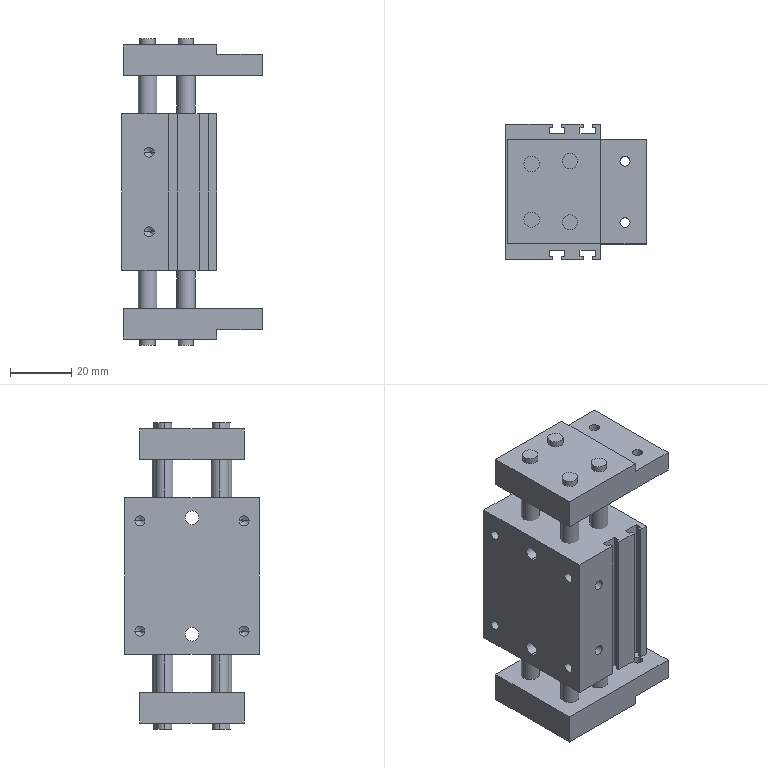Part | STEP file | MHL2-10D_Open | 3 solids | 146 faces | box 46 x 44 x 100 mm | volume 98131 mm3 | plane 70 | cylinder 60 | cone 16 | commonest cylinder face diameters 3.3 x20 5 x16 6 x16 4.2 x4 4.5 x4